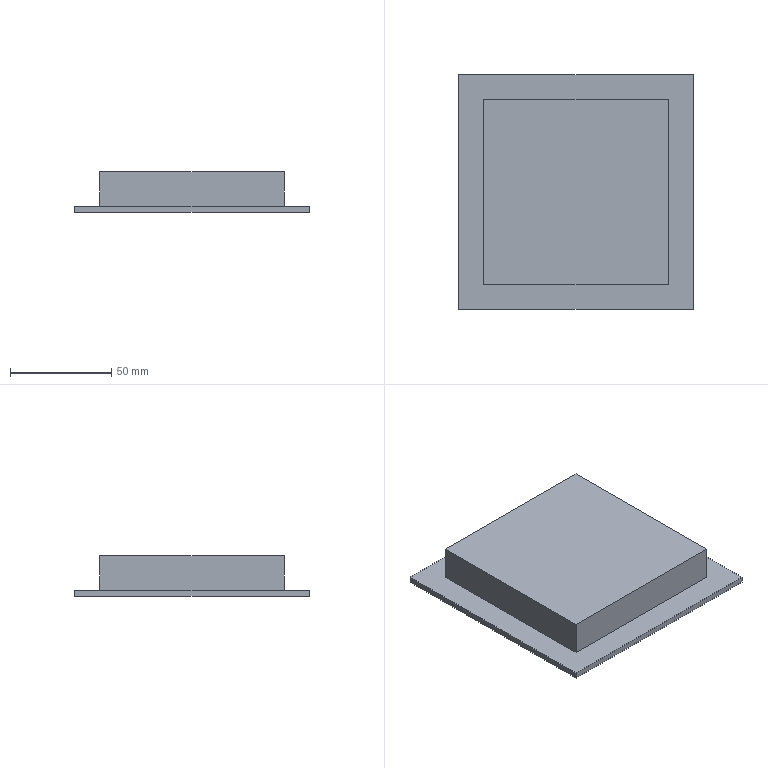Part | SolidWorks | features Extrusion 1, ICE 1 | 1 solid | 11 faces | box 116 x 116 x 20 mm | volume 181145 mm3 | plane 11
STEP:
#1=CARTESIAN_POINT('',(58.,-58.,0.));
#2=VERTEX_POINT('',#1);
#3=CARTESIAN_POINT('',(58.,58.,0.));
#4=VERTEX_POINT('',#3);
#5=CARTESIAN_POINT('',(58.,58.,0.));
#6=DIRECTION('',(0.,1.,0.));
#7=VECTOR('',#6,1000.);
#8=LINE('',#5,#7);
#9=EDGE_CURVE('',#2,#4,#8,.T.);
#10=ORIENTED_EDGE('',*,*,#9,.T.);
#11=CARTESIAN_POINT('',(58.,58.,3.));
#12=VERTEX_POINT('',#11);
#13=CARTESIAN_POINT('',(58.,58.,3.));
#14=DIRECTION('',(0.,0.,-1.));
#15=VECTOR('',#14,1000.);
#16=LINE('',#13,#15);
#17=EDGE_CURVE('',#12,#4,#16,.T.);
#18=ORIENTED_EDGE('',*,*,#17,.F.);
#19=CARTESIAN_POINT('',(58.,-58.,3.));
#20=VERTEX_POINT('',#19);
#21=CARTESIAN_POINT('',(58.,58.,3.));
#22=DIRECTION('',(0.,1.,0.));
#23=VECTOR('',#22,1000.);
#24=LINE('',#21,#23);
#25=EDGE_CURVE('',#20,#12,#24,.T.);
#26=ORIENTED_EDGE('',*,*,#25,.F.);
#27=CARTESIAN_POINT('',(58.,-58.,3.));
#28=DIRECTION('',(0.,0.,-1.));
#29=VECTOR('',#28,1000.);
#30=LINE('',#27,#29);
#31=EDGE_CURVE('',#20,#2,#30,.T.);
#32=ORIENTED_EDGE('',*,*,#31,.T.);
#33=EDGE_LOOP('',(#10,#18,#26,#32));
#34=FACE_OUTER_BOUND('',#33,.T.);
#35=CARTESIAN_POINT('',(58.,58.,3.));
#36=DIRECTION('',(-1.,0.,0.));
#37=DIRECTION('',(0.,-1.,0.));
#38=AXIS2_PLACEMENT_3D('',#35,#36,#37);
#39=PLANE('',#38);
#40=ADVANCED_FACE('',(#34),#39,.F.);
#41=CARTESIAN_POINT('',(-58.,58.,0.));
#42=VERTEX_POINT('',#41);
#43=CARTESIAN_POINT('',(-58.,58.,0.));
#44=DIRECTION('',(-1.,0.,0.));
#45=VECTOR('',#44,1000.);
#46=LINE('',#43,#45);
#47=EDGE_CURVE('',#4,#42,#46,.T.);
#48=ORIENTED_EDGE('',*,*,#47,.T.);
#49=CARTESIAN_POINT('',(-58.,58.,3.));
#50=VERTEX_POINT('',#49);
#51=CARTESIAN_POINT('',(-58.,58.,3.));
#52=DIRECTION('',(0.,0.,-1.));
#53=VECTOR('',#52,1000.);
#54=LINE('',#51,#53);
#55=EDGE_CURVE('',#50,#42,#54,.T.);
#56=ORIENTED_EDGE('',*,*,#55,.F.);
#57=CARTESIAN_POINT('',(-58.,58.,3.));
#58=DIRECTION('',(-1.,0.,0.));
#59=VECTOR('',#58,1000.);
#60=LINE('',#57,#59);
#61=EDGE_CURVE('',#12,#50,#60,.T.);
#62=ORIENTED_EDGE('',*,*,#61,.F.);
#63=ORIENTED_EDGE('',*,*,#17,.T.);
#64=EDGE_LOOP('',(#48,#56,#62,#63));
#65=FACE_OUTER_BOUND('',#64,.T.);
#66=CARTESIAN_POINT('',(-58.,58.,3.));
#67=DIRECTION('',(0.,-1.,0.));
#68=DIRECTION('',(0.,0.,-1.));
#69=AXIS2_PLACEMENT_3D('',#66,#67,#68);
#70=PLANE('',#69);
#71=ADVANCED_FACE('',(#65),#70,.F.);
#72=CARTESIAN_POINT('',(-58.,-58.,0.));
#73=VERTEX_POINT('',#72);
#74=CARTESIAN_POINT('',(-58.,58.,0.));
#75=DIRECTION('',(0.,-1.,0.));
#76=VECTOR('',#75,1000.);
#77=LINE('',#74,#76);
#78=EDGE_CURVE('',#42,#73,#77,.T.);
#79=ORIENTED_EDGE('',*,*,#78,.T.);
#80=CARTESIAN_POINT('',(-58.,-58.,3.));
#81=VERTEX_POINT('',#80);
#82=CARTESIAN_POINT('',(-58.,-58.,3.));
#83=DIRECTION('',(0.,0.,-1.));
#84=VECTOR('',#83,1000.);
#85=LINE('',#82,#84);
#86=EDGE_CURVE('',#81,#73,#85,.T.);
#87=ORIENTED_EDGE('',*,*,#86,.F.);
#88=CARTESIAN_POINT('',(-58.,58.,3.));
#89=DIRECTION('',(0.,-1.,0.));
#90=VECTOR('',#89,1000.);
#91=LINE('',#88,#90);
#92=EDGE_CURVE('',#50,#81,#91,.T.);
#93=ORIENTED_EDGE('',*,*,#92,.F.);
#94=ORIENTED_EDGE('',*,*,#55,.T.);
#95=EDGE_LOOP('',(#79,#87,#93,#94));
#96=FACE_OUTER_BOUND('',#95,.T.);
#97=CARTESIAN_POINT('',(-58.,58.,3.));
#98=DIRECTION('',(1.,0.,0.));
#99=DIRECTION('',(0.,1.,0.));
#100=AXIS2_PLACEMENT_3D('',#97,#98,#99);
#101=PLANE('',#100);
#102=ADVANCED_FACE('',(#96),#101,.F.);
#103=CARTESIAN_POINT('',(-58.,-58.,0.));
#104=DIRECTION('',(1.,0.,0.));
#105=VECTOR('',#104,1000.);
#106=LINE('',#103,#105);
#107=EDGE_CURVE('',#73,#2,#106,.T.);
#108=ORIENTED_EDGE('',*,*,#107,.T.);
#109=ORIENTED_EDGE('',*,*,#31,.F.);
#110=CARTESIAN_POINT('',(-58.,-58.,3.));
#111=DIRECTION('',(1.,0.,0.));
#112=VECTOR('',#111,1000.);
#113=LINE('',#110,#112);
#114=EDGE_CURVE('',#81,#20,#113,.T.);
#115=ORIENTED_EDGE('',*,*,#114,.F.);
#116=ORIENTED_EDGE('',*,*,#86,.T.);
#117=EDGE_LOOP('',(#108,#109,#115,#116));
#118=FACE_OUTER_BOUND('',#117,.T.);
#119=CARTESIAN_POINT('',(-58.,-58.,3.));
#120=DIRECTION('',(0.,1.,0.));
#121=DIRECTION('',(0.,0.,1.));
#122=AXIS2_PLACEMENT_3D('',#119,#120,#121);
#123=PLANE('',#122);
#124=ADVANCED_FACE('',(#118),#123,.F.);
#125=CARTESIAN_POINT('',(45.5,-45.5,3.));
#126=VERTEX_POINT('',#125);
#127=CARTESIAN_POINT('',(45.5,45.5,3.));
#128=VERTEX_POINT('',#127);
#129=CARTESIAN_POINT('',(45.5,45.5,3.));
#130=DIRECTION('',(0.,1.,0.));
#131=VECTOR('',#130,1000.);
#132=LINE('',#129,#131);
#133=EDGE_CURVE('',#126,#128,#132,.T.);
#134=ORIENTED_EDGE('',*,*,#133,.F.);
#135=CARTESIAN_POINT('',(-45.5,-45.5,3.));
#136=VERTEX_POINT('',#135);
#137=CARTESIAN_POINT('',(-45.5,-45.5,3.));
#138=DIRECTION('',(1.,0.,0.));
#139=VECTOR('',#138,1000.);
#140=LINE('',#137,#139);
#141=EDGE_CURVE('',#136,#126,#140,.T.);
#142=ORIENTED_EDGE('',*,*,#141,.F.);
#143=CARTESIAN_POINT('',(-45.5,45.5,3.));
#144=VERTEX_POINT('',#143);
#145=CARTESIAN_POINT('',(-45.5,45.5,3.));
#146=DIRECTION('',(0.,-1.,0.));
#147=VECTOR('',#146,1000.);
#148=LINE('',#145,#147);
#149=EDGE_CURVE('',#144,#136,#148,.T.);
#150=ORIENTED_EDGE('',*,*,#149,.F.);
#151=CARTESIAN_POINT('',(-45.5,45.5,3.));
#152=DIRECTION('',(-1.,0.,0.));
#153=VECTOR('',#152,1000.);
#154=LINE('',#151,#153);
#155=EDGE_CURVE('',#128,#144,#154,.T.);
#156=ORIENTED_EDGE('',*,*,#155,.F.);
#157=EDGE_LOOP('',(#134,#142,#150,#156));
#158=FACE_BOUND('',#157,.T.);
#159=ORIENTED_EDGE('',*,*,#25,.T.);
#160=ORIENTED_EDGE('',*,*,#61,.T.);
#161=ORIENTED_EDGE('',*,*,#92,.T.);
#162=ORIENTED_EDGE('',*,*,#114,.T.);
#163=EDGE_LOOP('',(#159,#160,#161,#162));
#164=FACE_OUTER_BOUND('',#163,.T.);
#165=CARTESIAN_POINT('',(0.,0.,3.));
#166=DIRECTION('',(0.,0.,1.));
#167=DIRECTION('',(1.,0.,0.));
#168=AXIS2_PLACEMENT_3D('',#165,#166,#167);
#169=PLANE('',#168);
#170=ADVANCED_FACE('',(#158,#164),#169,.T.);
#171=ORIENTED_EDGE('',*,*,#9,.F.);
#172=ORIENTED_EDGE('',*,*,#107,.F.);
#173=ORIENTED_EDGE('',*,*,#78,.F.);
#174=ORIENTED_EDGE('',*,*,#47,.F.);
#175=EDGE_LOOP('',(#171,#172,#173,#174));
#176=FACE_OUTER_BOUND('',#175,.T.);
#177=CARTESIAN_POINT('',(0.,0.,0.));
#178=DIRECTION('',(0.,0.,1.));
#179=DIRECTION('',(1.,0.,0.));
#180=AXIS2_PLACEMENT_3D('',#177,#178,#179);
#181=PLANE('',#180);
#182=ADVANCED_FACE('',(#176),#181,.F.);
#183=ORIENTED_EDGE('',*,*,#133,.T.);
#184=CARTESIAN_POINT('',(45.5,45.5,20.));
#185=VERTEX_POINT('',#184);
#186=CARTESIAN_POINT('',(45.5,45.5,20.));
#187=DIRECTION('',(0.,0.,-1.));
#188=VECTOR('',#187,1000.);
#189=LINE('',#186,#188);
#190=EDGE_CURVE('',#185,#128,#189,.T.);
#191=ORIENTED_EDGE('',*,*,#190,.F.);
#192=CARTESIAN_POINT('',(45.5,-45.5,20.));
#193=VERTEX_POINT('',#192);
#194=CARTESIAN_POINT('',(45.5,45.5,20.));
#195=DIRECTION('',(0.,1.,0.));
#196=VECTOR('',#195,1000.);
#197=LINE('',#194,#196);
#198=EDGE_CURVE('',#193,#185,#197,.T.);
#199=ORIENTED_EDGE('',*,*,#198,.F.);
#200=CARTESIAN_POINT('',(45.5,-45.5,20.));
#201=DIRECTION('',(0.,0.,-1.));
#202=VECTOR('',#201,1000.);
#203=LINE('',#200,#202);
#204=EDGE_CURVE('',#193,#126,#203,.T.);
#205=ORIENTED_EDGE('',*,*,#204,.T.);
#206=EDGE_LOOP('',(#183,#191,#199,#205));
#207=FACE_OUTER_BOUND('',#206,.T.);
#208=CARTESIAN_POINT('',(45.5,45.5,20.));
#209=DIRECTION('',(-1.,0.,0.));
#210=DIRECTION('',(0.,-1.,0.));
#211=AXIS2_PLACEMENT_3D('',#208,#209,#210);
#212=PLANE('',#211);
#213=ADVANCED_FACE('',(#207),#212,.F.);
#214=ORIENTED_EDGE('',*,*,#155,.T.);
#215=CARTESIAN_POINT('',(-45.5,45.5,20.));
#216=VERTEX_POINT('',#215);
#217=CARTESIAN_POINT('',(-45.5,45.5,20.));
#218=DIRECTION('',(0.,0.,-1.));
#219=VECTOR('',#218,1000.);
#220=LINE('',#217,#219);
#221=EDGE_CURVE('',#216,#144,#220,.T.);
#222=ORIENTED_EDGE('',*,*,#221,.F.);
#223=CARTESIAN_POINT('',(-45.5,45.5,20.));
#224=DIRECTION('',(-1.,0.,0.));
#225=VECTOR('',#224,1000.);
#226=LINE('',#223,#225);
#227=EDGE_CURVE('',#185,#216,#226,.T.);
#228=ORIENTED_EDGE('',*,*,#227,.F.);
#229=ORIENTED_EDGE('',*,*,#190,.T.);
#230=EDGE_LOOP('',(#214,#222,#228,#229));
#231=FACE_OUTER_BOUND('',#230,.T.);
#232=CARTESIAN_POINT('',(-45.5,45.5,20.));
#233=DIRECTION('',(0.,-1.,0.));
#234=DIRECTION('',(0.,0.,-1.));
#235=AXIS2_PLACEMENT_3D('',#232,#233,#234);
#236=PLANE('',#235);
#237=ADVANCED_FACE('',(#231),#236,.F.);
#238=ORIENTED_EDGE('',*,*,#149,.T.);
#239=CARTESIAN_POINT('',(-45.5,-45.5,20.));
#240=VERTEX_POINT('',#239);
#241=CARTESIAN_POINT('',(-45.5,-45.5,20.));
#242=DIRECTION('',(0.,0.,-1.));
#243=VECTOR('',#242,1000.);
#244=LINE('',#241,#243);
#245=EDGE_CURVE('',#240,#136,#244,.T.);
#246=ORIENTED_EDGE('',*,*,#245,.F.);
#247=CARTESIAN_POINT('',(-45.5,45.5,20.));
#248=DIRECTION('',(0.,-1.,0.));
#249=VECTOR('',#248,1000.);
#250=LINE('',#247,#249);
#251=EDGE_CURVE('',#216,#240,#250,.T.);
#252=ORIENTED_EDGE('',*,*,#251,.F.);
#253=ORIENTED_EDGE('',*,*,#221,.T.);
#254=EDGE_LOOP('',(#238,#246,#252,#253));
#255=FACE_OUTER_BOUND('',#254,.T.);
#256=CARTESIAN_POINT('',(-45.5,45.5,20.));
#257=DIRECTION('',(1.,0.,0.));
#258=DIRECTION('',(0.,1.,0.));
#259=AXIS2_PLACEMENT_3D('',#256,#257,#258);
#260=PLANE('',#259);
#261=ADVANCED_FACE('',(#255),#260,.F.);
#262=ORIENTED_EDGE('',*,*,#141,.T.);
#263=ORIENTED_EDGE('',*,*,#204,.F.);
#264=CARTESIAN_POINT('',(-45.5,-45.5,20.));
#265=DIRECTION('',(1.,0.,0.));
#266=VECTOR('',#265,1000.);
#267=LINE('',#264,#266);
#268=EDGE_CURVE('',#240,#193,#267,.T.);
#269=ORIENTED_EDGE('',*,*,#268,.F.);
#270=ORIENTED_EDGE('',*,*,#245,.T.);
#271=EDGE_LOOP('',(#262,#263,#269,#270));
#272=FACE_OUTER_BOUND('',#271,.T.);
#273=CARTESIAN_POINT('',(-45.5,-45.5,20.));
#274=DIRECTION('',(0.,1.,0.));
#275=DIRECTION('',(0.,0.,1.));
#276=AXIS2_PLACEMENT_3D('',#273,#274,#275);
#277=PLANE('',#276);
#278=ADVANCED_FACE('',(#272),#277,.F.);
#279=ORIENTED_EDGE('',*,*,#198,.T.);
#280=ORIENTED_EDGE('',*,*,#227,.T.);
#281=ORIENTED_EDGE('',*,*,#251,.T.);
#282=ORIENTED_EDGE('',*,*,#268,.T.);
#283=EDGE_LOOP('',(#279,#280,#281,#282));
#284=FACE_OUTER_BOUND('',#283,.T.);
#285=CARTESIAN_POINT('',(0.,0.,20.));
#286=DIRECTION('',(0.,0.,1.));
#287=DIRECTION('',(1.,0.,0.));
#288=AXIS2_PLACEMENT_3D('',#285,#286,#287);
#289=PLANE('',#288);
#290=ADVANCED_FACE('',(#284),#289,.T.);
#291=CLOSED_SHELL('',(#40,#71,#102,#124,#170,#182,#213,#237,#261,#278,#290));
#292=MANIFOLD_SOLID_BREP('',#291);
#293=CARTESIAN_POINT('',(0.,0.,0.));
#294=DIRECTION('',(0.,0.,1.));
#295=DIRECTION('',(1.,0.,0.));
#296=AXIS2_PLACEMENT_3D('',#293,#294,#295);
#297=(LENGTH_UNIT()NAMED_UNIT(*)SI_UNIT(.MILLI.,.METRE.));
#298=UNCERTAINTY_MEASURE_WITH_UNIT(LENGTH_MEASURE(0.00001),#297,'','');
#299=(NAMED_UNIT(*)PLANE_ANGLE_UNIT()SI_UNIT($,.RADIAN.));
#300=(NAMED_UNIT(*)SI_UNIT($,.STERADIAN.)SOLID_ANGLE_UNIT());
#301=(GEOMETRIC_REPRESENTATION_CONTEXT(3)GLOBAL_UNCERTAINTY_ASSIGNED_CONTEXT((#298))GLOBAL_UNIT_ASSIGNED_CONTEXT((#297,#299,#300))REPRESENTATION_CONTEXT('',''));
#302=ADVANCED_BREP_SHAPE_REPRESENTATION('',(#292,#296),#301);